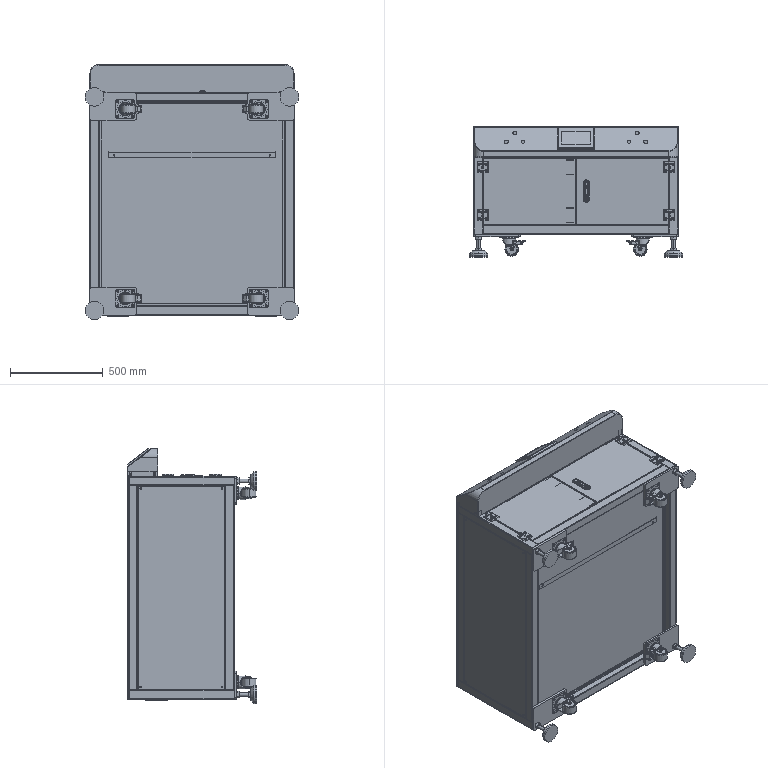Part | SolidWorks | features InContextFeatHolder 16, ReferencePattern 13, MirrorCompFeat 5 | 159 solids | 4925 faces | volume 25832975 mm3 | cylinder 1982 | plane 1736 | cone 485 | spline 383 | torus 303 | sphere 36 | commonest cylinder face diameters 1 x210 8 x200 5 x136 10 x132 4 x127 6 x103